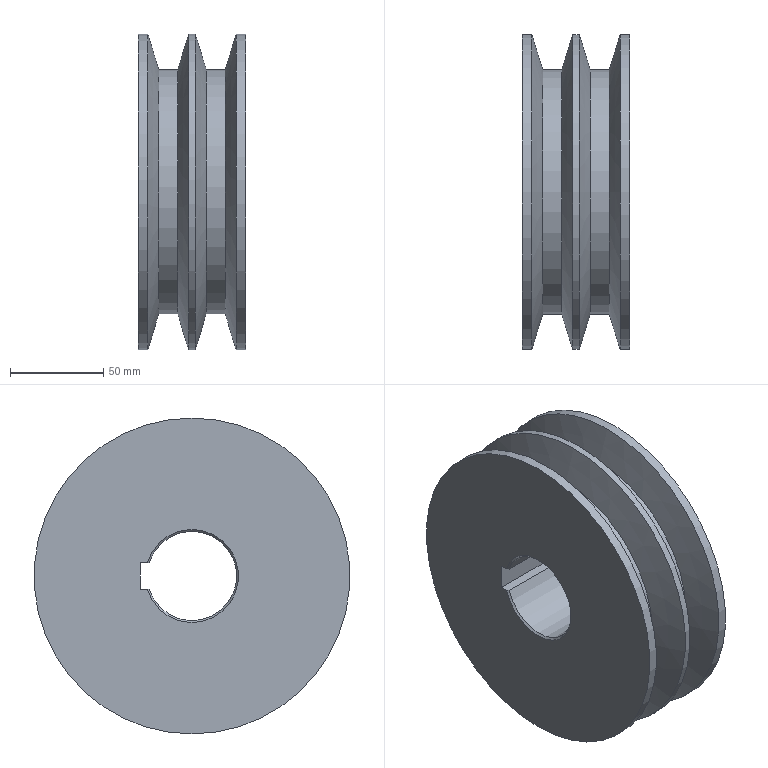Part | NX | features 小带轮_实心轮 2 | 1 solid | 19 faces | box 57.5 x 169.6 x 169.6 mm | volume 872615 mm3 | cylinder 7 | plane 6 | cone 6 | commonest cylinder face diameters 169.6 x3 131.4 x2 48 x1 80 x1
STEP:
#1=CARTESIAN_POINT('',(57.5,0.,84.8));
#2=VERTEX_POINT('',#1);
#3=CARTESIAN_POINT('',(57.5,0.,0.));
#4=DIRECTION('',(-1.,0.,0.));
#5=DIRECTION('',(0.,0.,1.));
#6=AXIS2_PLACEMENT_3D('',#3,#4,#5);
#7=CIRCLE('',#6,84.8);
#8=EDGE_CURVE('',#2,#2,#7,.T.);
#9=ORIENTED_EDGE('',*,*,#8,.T.);
#10=EDGE_LOOP('',(#9));
#11=FACE_BOUND('',#10,.T.);
#12=CARTESIAN_POINT('',(52.468,0.,84.8));
#13=VERTEX_POINT('',#12);
#14=CARTESIAN_POINT('',(52.468,0.,0.));
#15=DIRECTION('',(-1.,0.,0.));
#16=DIRECTION('',(0.,0.,1.));
#17=AXIS2_PLACEMENT_3D('',#14,#15,#16);
#18=CIRCLE('',#17,84.8);
#19=EDGE_CURVE('',#13,#13,#18,.T.);
#20=ORIENTED_EDGE('',*,*,#19,.F.);
#21=EDGE_LOOP('',(#20));
#22=FACE_BOUND('',#21,.T.);
#23=CARTESIAN_POINT('',(0.,0.,0.));
#24=DIRECTION('',(-1.,0.,0.));
#25=DIRECTION('',(0.,0.,1.));
#26=AXIS2_PLACEMENT_3D('',#23,#24,#25);
#27=CYLINDRICAL_SURFACE('',#26,84.8);
#28=ADVANCED_FACE('',(#11,#22),#27,.T.);
#29=CARTESIAN_POINT('',(26.968,0.,84.8));
#30=VERTEX_POINT('',#29);
#31=CARTESIAN_POINT('',(26.968,0.,0.));
#32=DIRECTION('',(-1.,0.,0.));
#33=DIRECTION('',(0.,0.,1.));
#34=AXIS2_PLACEMENT_3D('',#31,#32,#33);
#35=CIRCLE('',#34,84.8);
#36=EDGE_CURVE('',#30,#30,#35,.T.);
#37=ORIENTED_EDGE('',*,*,#36,.F.);
#38=EDGE_LOOP('',(#37));
#39=FACE_BOUND('',#38,.T.);
#40=CARTESIAN_POINT('',(30.532,0.,84.8));
#41=VERTEX_POINT('',#40);
#42=CARTESIAN_POINT('',(30.532,0.,0.));
#43=DIRECTION('',(-1.,0.,0.));
#44=DIRECTION('',(0.,0.,1.));
#45=AXIS2_PLACEMENT_3D('',#42,#43,#44);
#46=CIRCLE('',#45,84.8);
#47=EDGE_CURVE('',#41,#41,#46,.T.);
#48=ORIENTED_EDGE('',*,*,#47,.T.);
#49=EDGE_LOOP('',(#48));
#50=FACE_BOUND('',#49,.T.);
#51=CARTESIAN_POINT('',(0.,0.,0.));
#52=DIRECTION('',(-1.,0.,0.));
#53=DIRECTION('',(0.,0.,1.));
#54=AXIS2_PLACEMENT_3D('',#51,#52,#53);
#55=CYLINDRICAL_SURFACE('',#54,84.8);
#56=ADVANCED_FACE('',(#39,#50),#55,.T.);
#57=CARTESIAN_POINT('',(0.,0.,84.8));
#58=VERTEX_POINT('',#57);
#59=CARTESIAN_POINT('',(0.,0.,0.));
#60=DIRECTION('',(-1.,0.,0.));
#61=DIRECTION('',(0.,0.,1.));
#62=AXIS2_PLACEMENT_3D('',#59,#60,#61);
#63=CIRCLE('',#62,84.8);
#64=EDGE_CURVE('',#58,#58,#63,.T.);
#65=ORIENTED_EDGE('',*,*,#64,.F.);
#66=EDGE_LOOP('',(#65));
#67=FACE_BOUND('',#66,.T.);
#68=CARTESIAN_POINT('',(5.032,0.,84.8));
#69=VERTEX_POINT('',#68);
#70=CARTESIAN_POINT('',(5.032,0.,0.));
#71=DIRECTION('',(-1.,0.,0.));
#72=DIRECTION('',(0.,0.,1.));
#73=AXIS2_PLACEMENT_3D('',#70,#71,#72);
#74=CIRCLE('',#73,84.8);
#75=EDGE_CURVE('',#69,#69,#74,.T.);
#76=ORIENTED_EDGE('',*,*,#75,.T.);
#77=EDGE_LOOP('',(#76));
#78=FACE_BOUND('',#77,.T.);
#79=CARTESIAN_POINT('',(0.,0.,0.));
#80=DIRECTION('',(-1.,0.,0.));
#81=DIRECTION('',(0.,0.,1.));
#82=AXIS2_PLACEMENT_3D('',#79,#80,#81);
#83=CYLINDRICAL_SURFACE('',#82,84.8);
#84=ADVANCED_FACE('',(#67,#78),#83,.T.);
#85=CARTESIAN_POINT('',(1.,22.956,-7.));
#86=VERTEX_POINT('',#85);
#87=CARTESIAN_POINT('',(1.,22.956,7.));
#88=VERTEX_POINT('',#87);
#89=CARTESIAN_POINT('',(1.,0.,0.));
#90=DIRECTION('',(1.,0.,0.));
#91=DIRECTION('',(0.,0.,-1.));
#92=AXIS2_PLACEMENT_3D('',#89,#90,#91);
#93=CIRCLE('',#92,24.);
#94=EDGE_CURVE('',#86,#88,#93,.F.);
#95=ORIENTED_EDGE('',*,*,#94,.T.);
#96=CARTESIAN_POINT('',(49.,22.956,7.));
#97=VERTEX_POINT('',#96);
#98=CARTESIAN_POINT('',(57.5,22.956,7.));
#99=DIRECTION('',(-1.,0.,0.));
#100=VECTOR('',#99,1000.);
#101=LINE('',#98,#100);
#102=EDGE_CURVE('',#97,#88,#101,.T.);
#103=ORIENTED_EDGE('',*,*,#102,.F.);
#104=CARTESIAN_POINT('',(49.,22.956,-7.));
#105=VERTEX_POINT('',#104);
#106=CARTESIAN_POINT('',(49.,0.,0.));
#107=DIRECTION('',(-1.,0.,0.));
#108=DIRECTION('',(0.,0.,1.));
#109=AXIS2_PLACEMENT_3D('',#106,#107,#108);
#110=CIRCLE('',#109,24.);
#111=EDGE_CURVE('',#97,#105,#110,.F.);
#112=ORIENTED_EDGE('',*,*,#111,.T.);
#113=CARTESIAN_POINT('',(57.5,22.956,-7.));
#114=DIRECTION('',(-1.,0.,0.));
#115=VECTOR('',#114,1000.);
#116=LINE('',#113,#115);
#117=EDGE_CURVE('',#105,#86,#116,.T.);
#118=ORIENTED_EDGE('',*,*,#117,.T.);
#119=EDGE_LOOP('',(#95,#103,#112,#118));
#120=FACE_BOUND('',#119,.T.);
#121=CARTESIAN_POINT('',(0.,0.,0.));
#122=DIRECTION('',(-1.,0.,0.));
#123=DIRECTION('',(0.,0.,1.));
#124=AXIS2_PLACEMENT_3D('',#121,#122,#123);
#125=CYLINDRICAL_SURFACE('',#124,24.);
#126=ADVANCED_FACE('',(#120),#125,.F.);
#127=CARTESIAN_POINT('',(50.,27.8,7.));
#128=VERTEX_POINT('',#127);
#129=CARTESIAN_POINT('',(50.,27.8,-7.));
#130=VERTEX_POINT('',#129);
#131=CARTESIAN_POINT('',(50.,27.8,0.));
#132=DIRECTION('',(0.,0.,-1.));
#133=VECTOR('',#132,1000.);
#134=LINE('',#131,#133);
#135=EDGE_CURVE('',#128,#130,#134,.T.);
#136=ORIENTED_EDGE('',*,*,#135,.T.);
#137=CARTESIAN_POINT('',(50.,24.,-7.));
#138=VERTEX_POINT('',#137);
#139=CARTESIAN_POINT('',(50.,40.,-7.));
#140=DIRECTION('',(0.,-1.,0.));
#141=VECTOR('',#140,1000.);
#142=LINE('',#139,#141);
#143=EDGE_CURVE('',#130,#138,#142,.T.);
#144=ORIENTED_EDGE('',*,*,#143,.T.);
#145=CARTESIAN_POINT('',(50.,24.,7.));
#146=VERTEX_POINT('',#145);
#147=CARTESIAN_POINT('',(50.,0.,0.));
#148=DIRECTION('',(-1.,0.,0.));
#149=DIRECTION('',(0.,0.,1.));
#150=AXIS2_PLACEMENT_3D('',#147,#148,#149);
#151=CIRCLE('',#150,25.);
#152=EDGE_CURVE('',#138,#146,#151,.T.);
#153=ORIENTED_EDGE('',*,*,#152,.T.);
#154=CARTESIAN_POINT('',(50.,40.,7.));
#155=DIRECTION('',(0.,1.,0.));
#156=VECTOR('',#155,1000.);
#157=LINE('',#154,#156);
#158=EDGE_CURVE('',#146,#128,#157,.T.);
#159=ORIENTED_EDGE('',*,*,#158,.T.);
#160=EDGE_LOOP('',(#136,#144,#153,#159));
#161=FACE_BOUND('',#160,.T.);
#162=CARTESIAN_POINT('',(50.,0.,40.));
#163=VERTEX_POINT('',#162);
#164=CARTESIAN_POINT('',(50.,0.,0.));
#165=DIRECTION('',(-1.,0.,0.));
#166=DIRECTION('',(0.,0.,1.));
#167=AXIS2_PLACEMENT_3D('',#164,#165,#166);
#168=CIRCLE('',#167,40.);
#169=EDGE_CURVE('',#163,#163,#168,.T.);
#170=ORIENTED_EDGE('',*,*,#169,.F.);
#171=EDGE_LOOP('',(#170));
#172=FACE_BOUND('',#171,.T.);
#173=CARTESIAN_POINT('',(50.,40.,0.));
#174=DIRECTION('',(-1.,0.,0.));
#175=DIRECTION('',(0.,0.,1.));
#176=AXIS2_PLACEMENT_3D('',#173,#174,#175);
#177=PLANE('',#176);
#178=ADVANCED_FACE('',(#161,#172),#177,.F.);
#179=CARTESIAN_POINT('',(57.5,0.,40.));
#180=VERTEX_POINT('',#179);
#181=CARTESIAN_POINT('',(57.5,0.,0.));
#182=DIRECTION('',(-1.,0.,0.));
#183=DIRECTION('',(0.,0.,1.));
#184=AXIS2_PLACEMENT_3D('',#181,#182,#183);
#185=CIRCLE('',#184,40.);
#186=EDGE_CURVE('',#180,#180,#185,.T.);
#187=ORIENTED_EDGE('',*,*,#186,.F.);
#188=EDGE_LOOP('',(#187));
#189=FACE_BOUND('',#188,.T.);
#190=ORIENTED_EDGE('',*,*,#169,.T.);
#191=EDGE_LOOP('',(#190));
#192=FACE_BOUND('',#191,.T.);
#193=CARTESIAN_POINT('',(0.,0.,0.));
#194=DIRECTION('',(-1.,0.,0.));
#195=DIRECTION('',(0.,0.,1.));
#196=AXIS2_PLACEMENT_3D('',#193,#194,#195);
#197=CYLINDRICAL_SURFACE('',#196,40.);
#198=ADVANCED_FACE('',(#189,#192),#197,.F.);
#199=ORIENTED_EDGE('',*,*,#8,.F.);
#200=EDGE_LOOP('',(#199));
#201=FACE_BOUND('',#200,.T.);
#202=ORIENTED_EDGE('',*,*,#186,.T.);
#203=EDGE_LOOP('',(#202));
#204=FACE_BOUND('',#203,.T.);
#205=CARTESIAN_POINT('',(57.5,84.8,0.));
#206=DIRECTION('',(-1.,0.,0.));
#207=DIRECTION('',(0.,0.,1.));
#208=AXIS2_PLACEMENT_3D('',#205,#206,#207);
#209=PLANE('',#208);
#210=ADVANCED_FACE('',(#201,#204),#209,.F.);
#211=CARTESIAN_POINT('',(0.,24.,7.));
#212=VERTEX_POINT('',#211);
#213=CARTESIAN_POINT('',(0.,24.,-7.));
#214=VERTEX_POINT('',#213);
#215=CARTESIAN_POINT('',(0.,0.,0.));
#216=DIRECTION('',(1.,0.,0.));
#217=DIRECTION('',(0.,0.,-1.));
#218=AXIS2_PLACEMENT_3D('',#215,#216,#217);
#219=CIRCLE('',#218,25.);
#220=EDGE_CURVE('',#212,#214,#219,.T.);
#221=ORIENTED_EDGE('',*,*,#220,.T.);
#222=CARTESIAN_POINT('',(0.,27.8,-7.));
#223=VERTEX_POINT('',#222);
#224=CARTESIAN_POINT('',(0.,22.956,-7.));
#225=DIRECTION('',(0.,-1.,0.));
#226=VECTOR('',#225,1000.);
#227=LINE('',#224,#226);
#228=EDGE_CURVE('',#223,#214,#227,.T.);
#229=ORIENTED_EDGE('',*,*,#228,.F.);
#230=CARTESIAN_POINT('',(0.,27.8,7.));
#231=VERTEX_POINT('',#230);
#232=CARTESIAN_POINT('',(0.,27.8,-7.));
#233=DIRECTION('',(0.,0.,-1.));
#234=VECTOR('',#233,1000.);
#235=LINE('',#232,#234);
#236=EDGE_CURVE('',#231,#223,#235,.T.);
#237=ORIENTED_EDGE('',*,*,#236,.F.);
#238=CARTESIAN_POINT('',(0.,22.956,7.));
#239=DIRECTION('',(0.,1.,0.));
#240=VECTOR('',#239,1000.);
#241=LINE('',#238,#240);
#242=EDGE_CURVE('',#212,#231,#241,.T.);
#243=ORIENTED_EDGE('',*,*,#242,.F.);
#244=EDGE_LOOP('',(#221,#229,#237,#243));
#245=FACE_BOUND('',#244,.T.);
#246=ORIENTED_EDGE('',*,*,#64,.T.);
#247=EDGE_LOOP('',(#246));
#248=FACE_BOUND('',#247,.T.);
#249=CARTESIAN_POINT('',(0.,24.,0.));
#250=DIRECTION('',(1.,0.,0.));
#251=DIRECTION('',(0.,0.,-1.));
#252=AXIS2_PLACEMENT_3D('',#249,#250,#251);
#253=PLANE('',#252);
#254=ADVANCED_FACE('',(#245,#248),#253,.F.);
#255=CARTESIAN_POINT('',(21.128,0.,65.7));
#256=VERTEX_POINT('',#255);
#257=CARTESIAN_POINT('',(21.128,0.,0.));
#258=DIRECTION('',(-1.,0.,0.));
#259=DIRECTION('',(0.,0.,1.));
#260=AXIS2_PLACEMENT_3D('',#257,#258,#259);
#261=CIRCLE('',#260,65.7);
#262=EDGE_CURVE('',#256,#256,#261,.T.);
#263=ORIENTED_EDGE('',*,*,#262,.T.);
#264=EDGE_LOOP('',(#263));
#265=FACE_BOUND('',#264,.T.);
#266=CARTESIAN_POINT('',(10.872,0.,65.7));
#267=VERTEX_POINT('',#266);
#268=CARTESIAN_POINT('',(10.872,0.,0.));
#269=DIRECTION('',(-1.,0.,0.));
#270=DIRECTION('',(0.,0.,1.));
#271=AXIS2_PLACEMENT_3D('',#268,#269,#270);
#272=CIRCLE('',#271,65.7);
#273=EDGE_CURVE('',#267,#267,#272,.T.);
#274=ORIENTED_EDGE('',*,*,#273,.F.);
#275=EDGE_LOOP('',(#274));
#276=FACE_BOUND('',#275,.T.);
#277=CARTESIAN_POINT('',(0.,0.,0.));
#278=DIRECTION('',(-1.,0.,0.));
#279=DIRECTION('',(0.,0.,1.));
#280=AXIS2_PLACEMENT_3D('',#277,#278,#279);
#281=CYLINDRICAL_SURFACE('',#280,65.7);
#282=ADVANCED_FACE('',(#265,#276),#281,.T.);
#283=ORIENTED_EDGE('',*,*,#36,.T.);
#284=EDGE_LOOP('',(#283));
#285=FACE_BOUND('',#284,.T.);
#286=ORIENTED_EDGE('',*,*,#262,.F.);
#287=EDGE_LOOP('',(#286));
#288=FACE_BOUND('',#287,.T.);
#289=CARTESIAN_POINT('',(21.128,0.,0.));
#290=DIRECTION('',(1.,0.,0.));
#291=DIRECTION('',(0.,0.,-1.));
#292=AXIS2_PLACEMENT_3D('',#289,#290,#291);
#293=CONICAL_SURFACE('',#292,65.7,1.274);
#294=ADVANCED_FACE('',(#285,#288),#293,.T.);
#295=ORIENTED_EDGE('',*,*,#273,.T.);
#296=EDGE_LOOP('',(#295));
#297=FACE_BOUND('',#296,.T.);
#298=ORIENTED_EDGE('',*,*,#75,.F.);
#299=EDGE_LOOP('',(#298));
#300=FACE_BOUND('',#299,.T.);
#301=CARTESIAN_POINT('',(5.032,0.,0.));
#302=DIRECTION('',(-1.,0.,0.));
#303=DIRECTION('',(0.,0.,1.));
#304=AXIS2_PLACEMENT_3D('',#301,#302,#303);
#305=CONICAL_SURFACE('',#304,84.8,1.274);
#306=ADVANCED_FACE('',(#297,#300),#305,.T.);
#307=CARTESIAN_POINT('',(46.628,0.,65.7));
#308=VERTEX_POINT('',#307);
#309=CARTESIAN_POINT('',(46.628,0.,0.));
#310=DIRECTION('',(-1.,0.,0.));
#311=DIRECTION('',(0.,0.,1.));
#312=AXIS2_PLACEMENT_3D('',#309,#310,#311);
#313=CIRCLE('',#312,65.7);
#314=EDGE_CURVE('',#308,#308,#313,.T.);
#315=ORIENTED_EDGE('',*,*,#314,.T.);
#316=EDGE_LOOP('',(#315));
#317=FACE_BOUND('',#316,.T.);
#318=CARTESIAN_POINT('',(36.372,0.,65.7));
#319=VERTEX_POINT('',#318);
#320=CARTESIAN_POINT('',(36.372,0.,0.));
#321=DIRECTION('',(-1.,0.,0.));
#322=DIRECTION('',(0.,0.,1.));
#323=AXIS2_PLACEMENT_3D('',#320,#321,#322);
#324=CIRCLE('',#323,65.7);
#325=EDGE_CURVE('',#319,#319,#324,.T.);
#326=ORIENTED_EDGE('',*,*,#325,.F.);
#327=EDGE_LOOP('',(#326));
#328=FACE_BOUND('',#327,.T.);
#329=CARTESIAN_POINT('',(25.5,0.,0.));
#330=DIRECTION('',(-1.,0.,0.));
#331=DIRECTION('',(0.,0.,1.));
#332=AXIS2_PLACEMENT_3D('',#329,#330,#331);
#333=CYLINDRICAL_SURFACE('',#332,65.7);
#334=ADVANCED_FACE('',(#317,#328),#333,.T.);
#335=ORIENTED_EDGE('',*,*,#19,.T.);
#336=EDGE_LOOP('',(#335));
#337=FACE_BOUND('',#336,.T.);
#338=ORIENTED_EDGE('',*,*,#314,.F.);
#339=EDGE_LOOP('',(#338));
#340=FACE_BOUND('',#339,.T.);
#341=CARTESIAN_POINT('',(46.628,0.,0.));
#342=DIRECTION('',(1.,0.,0.));
#343=DIRECTION('',(0.,0.,-1.));
#344=AXIS2_PLACEMENT_3D('',#341,#342,#343);
#345=CONICAL_SURFACE('',#344,65.7,1.274);
#346=ADVANCED_FACE('',(#337,#340),#345,.T.);
#347=ORIENTED_EDGE('',*,*,#325,.T.);
#348=EDGE_LOOP('',(#347));
#349=FACE_BOUND('',#348,.T.);
#350=ORIENTED_EDGE('',*,*,#47,.F.);
#351=EDGE_LOOP('',(#350));
#352=FACE_BOUND('',#351,.T.);
#353=CARTESIAN_POINT('',(30.532,0.,0.));
#354=DIRECTION('',(-1.,0.,0.));
#355=DIRECTION('',(0.,0.,1.));
#356=AXIS2_PLACEMENT_3D('',#353,#354,#355);
#357=CONICAL_SURFACE('',#356,84.8,1.274);
#358=ADVANCED_FACE('',(#349,#352),#357,.T.);
#359=CARTESIAN_POINT('',(49.,22.956,-7.));
#360=CARTESIAN_POINT('',(49.333,23.305,-7.));
#361=CARTESIAN_POINT('',(49.666,23.652,-7.));
#362=CARTESIAN_POINT('',(50.,24.,-7.));
#363=B_SPLINE_CURVE_WITH_KNOTS('',3,(#359,#360,#361,#362),.UNSPECIFIED.,.F.,.F.,(4,4),(0.004167,0.005613),.UNSPECIFIED.);
#364=EDGE_CURVE('',#105,#138,#363,.T.);
#365=ORIENTED_EDGE('',*,*,#364,.F.);
#366=ORIENTED_EDGE('',*,*,#111,.F.);
#367=CARTESIAN_POINT('',(50.,24.,7.));
#368=CARTESIAN_POINT('',(49.666,23.652,7.));
#369=CARTESIAN_POINT('',(49.333,23.305,7.));
#370=CARTESIAN_POINT('',(49.,22.956,7.));
#371=B_SPLINE_CURVE_WITH_KNOTS('',3,(#367,#368,#369,#370),.UNSPECIFIED.,.F.,.F.,(4,4),(0.003437,0.004882),.UNSPECIFIED.);
#372=EDGE_CURVE('',#146,#97,#371,.T.);
#373=ORIENTED_EDGE('',*,*,#372,.F.);
#374=ORIENTED_EDGE('',*,*,#152,.F.);
#375=EDGE_LOOP('',(#365,#366,#373,#374));
#376=FACE_BOUND('',#375,.T.);
#377=CARTESIAN_POINT('',(50.,0.,0.));
#378=DIRECTION('',(1.,0.,0.));
#379=DIRECTION('',(0.,0.,-1.));
#380=AXIS2_PLACEMENT_3D('',#377,#378,#379);
#381=CONICAL_SURFACE('',#380,25.,0.7854);
#382=ADVANCED_FACE('',(#376),#381,.F.);
#383=CARTESIAN_POINT('',(0.,24.,-7.));
#384=CARTESIAN_POINT('',(0.3336,23.652,-7.));
#385=CARTESIAN_POINT('',(0.667,23.305,-7.));
#386=CARTESIAN_POINT('',(1.,22.956,-7.));
#387=B_SPLINE_CURVE_WITH_KNOTS('',3,(#383,#384,#385,#386),.UNSPECIFIED.,.F.,.F.,(4,4),(0.003437,0.004882),.UNSPECIFIED.);
#388=EDGE_CURVE('',#214,#86,#387,.T.);
#389=ORIENTED_EDGE('',*,*,#388,.F.);
#390=ORIENTED_EDGE('',*,*,#220,.F.);
#391=CARTESIAN_POINT('',(1.,22.956,7.));
#392=CARTESIAN_POINT('',(0.667,23.305,7.));
#393=CARTESIAN_POINT('',(0.3336,23.652,7.));
#394=CARTESIAN_POINT('',(0.,24.,7.));
#395=B_SPLINE_CURVE_WITH_KNOTS('',3,(#391,#392,#393,#394),.UNSPECIFIED.,.F.,.F.,(4,4),(0.004167,0.005613),.UNSPECIFIED.);
#396=EDGE_CURVE('',#88,#212,#395,.T.);
#397=ORIENTED_EDGE('',*,*,#396,.F.);
#398=ORIENTED_EDGE('',*,*,#94,.F.);
#399=EDGE_LOOP('',(#389,#390,#397,#398));
#400=FACE_BOUND('',#399,.T.);
#401=CARTESIAN_POINT('',(1.,0.,0.));
#402=DIRECTION('',(-1.,0.,0.));
#403=DIRECTION('',(0.,0.,1.));
#404=AXIS2_PLACEMENT_3D('',#401,#402,#403);
#405=CONICAL_SURFACE('',#404,24.,0.7854);
#406=ADVANCED_FACE('',(#400),#405,.F.);
#407=CARTESIAN_POINT('',(57.5,27.8,7.));
#408=DIRECTION('',(-1.,0.,0.));
#409=VECTOR('',#408,1000.);
#410=LINE('',#407,#409);
#411=EDGE_CURVE('',#128,#231,#410,.T.);
#412=ORIENTED_EDGE('',*,*,#411,.T.);
#413=ORIENTED_EDGE('',*,*,#236,.T.);
#414=CARTESIAN_POINT('',(57.5,27.8,-7.));
#415=DIRECTION('',(-1.,0.,0.));
#416=VECTOR('',#415,1000.);
#417=LINE('',#414,#416);
#418=EDGE_CURVE('',#130,#223,#417,.T.);
#419=ORIENTED_EDGE('',*,*,#418,.F.);
#420=ORIENTED_EDGE('',*,*,#135,.F.);
#421=EDGE_LOOP('',(#412,#413,#419,#420));
#422=FACE_BOUND('',#421,.T.);
#423=CARTESIAN_POINT('',(57.5,27.8,-7.));
#424=DIRECTION('',(0.,1.,0.));
#425=DIRECTION('',(0.,0.,1.));
#426=AXIS2_PLACEMENT_3D('',#423,#424,#425);
#427=PLANE('',#426);
#428=ADVANCED_FACE('',(#422),#427,.F.);
#429=ORIENTED_EDGE('',*,*,#418,.T.);
#430=ORIENTED_EDGE('',*,*,#228,.T.);
#431=ORIENTED_EDGE('',*,*,#388,.T.);
#432=ORIENTED_EDGE('',*,*,#117,.F.);
#433=ORIENTED_EDGE('',*,*,#364,.T.);
#434=ORIENTED_EDGE('',*,*,#143,.F.);
#435=EDGE_LOOP('',(#429,#430,#431,#432,#433,#434));
#436=FACE_BOUND('',#435,.T.);
#437=CARTESIAN_POINT('',(57.5,22.956,-7.));
#438=DIRECTION('',(0.,0.,-1.));
#439=DIRECTION('',(-1.,0.,0.));
#440=AXIS2_PLACEMENT_3D('',#437,#438,#439);
#441=PLANE('',#440);
#442=ADVANCED_FACE('',(#436),#441,.F.);
#443=ORIENTED_EDGE('',*,*,#372,.T.);
#444=ORIENTED_EDGE('',*,*,#102,.T.);
#445=ORIENTED_EDGE('',*,*,#396,.T.);
#446=ORIENTED_EDGE('',*,*,#242,.T.);
#447=ORIENTED_EDGE('',*,*,#411,.F.);
#448=ORIENTED_EDGE('',*,*,#158,.F.);
#449=EDGE_LOOP('',(#443,#444,#445,#446,#447,#448));
#450=FACE_BOUND('',#449,.T.);
#451=CARTESIAN_POINT('',(57.5,22.956,7.));
#452=DIRECTION('',(0.,0.,1.));
#453=DIRECTION('',(1.,0.,0.));
#454=AXIS2_PLACEMENT_3D('',#451,#452,#453);
#455=PLANE('',#454);
#456=ADVANCED_FACE('',(#450),#455,.F.);
#457=CLOSED_SHELL('',(#28,#56,#84,#126,#178,#198,#210,#254,#282,#294,#306,#334,#346,#358,#382,#406,#428,#442,#456));
#458=MANIFOLD_SOLID_BREP('',#457);
#459=(LENGTH_UNIT()NAMED_UNIT(*)SI_UNIT(.MILLI.,.METRE.));
#460=UNCERTAINTY_MEASURE_WITH_UNIT(LENGTH_MEASURE(0.0508),#459,'','');
#461=(NAMED_UNIT(*)PLANE_ANGLE_UNIT()SI_UNIT($,.RADIAN.));
#462=(NAMED_UNIT(*)SI_UNIT($,.STERADIAN.)SOLID_ANGLE_UNIT());
#463=(GEOMETRIC_REPRESENTATION_CONTEXT(3)GLOBAL_UNCERTAINTY_ASSIGNED_CONTEXT((#460))GLOBAL_UNIT_ASSIGNED_CONTEXT((#459,#461,#462))REPRESENTATION_CONTEXT('',''));
#464=ADVANCED_BREP_SHAPE_REPRESENTATION('',(#458),#463);